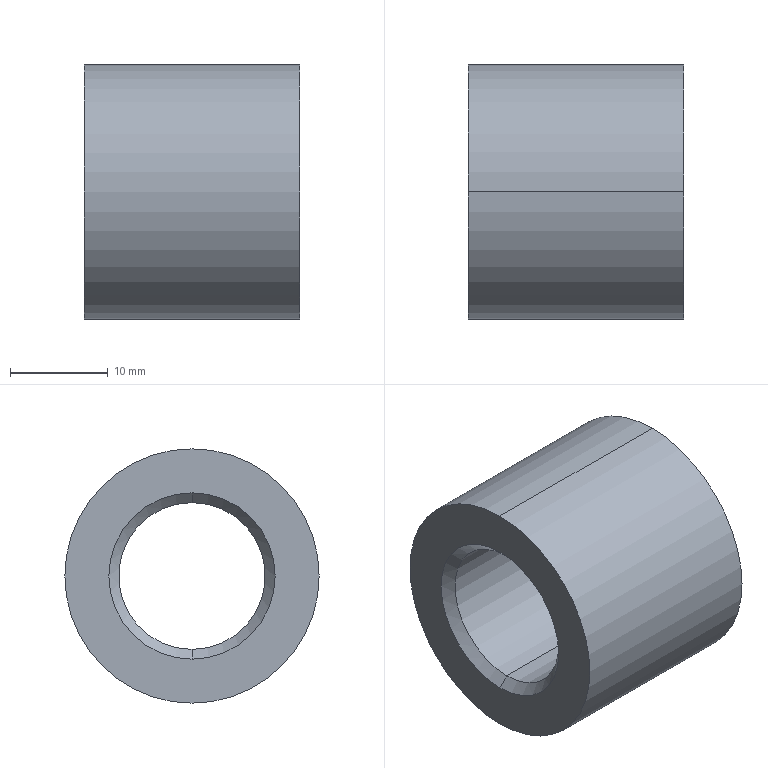Part | SolidWorks | features BaseBody 1 | 1 solid | 10 faces | box 22 x 26 x 26 mm | volume 7744 mm3 | cylinder 4 | cone 4 | plane 2 | commonest cylinder face diameters 15 x2 26 x2
STEP:
#1=CARTESIAN_POINT('',(22.,0.,-13.));
#2=VERTEX_POINT('',#1);
#3=CARTESIAN_POINT('',(22.,0.,13.));
#4=VERTEX_POINT('',#3);
#5=CARTESIAN_POINT('',(22.,0.,0.));
#6=DIRECTION('',(-1.,0.,0.));
#7=DIRECTION('',(0.,1.,0.));
#8=AXIS2_PLACEMENT_3D('',#5,#6,#7);
#9=CIRCLE('',#8,13.);
#10=EDGE_CURVE('',#2,#4,#9,.T.);
#11=ORIENTED_EDGE('',*,*,#10,.T.);
#12=CARTESIAN_POINT('',(0.,0.,13.));
#13=VERTEX_POINT('',#12);
#14=CARTESIAN_POINT('',(22.,0.,13.));
#15=DIRECTION('',(-1.,0.,0.));
#16=VECTOR('',#15,1000.);
#17=LINE('',#14,#16);
#18=EDGE_CURVE('',#4,#13,#17,.T.);
#19=ORIENTED_EDGE('',*,*,#18,.T.);
#20=CARTESIAN_POINT('',(0.,0.,-13.));
#21=VERTEX_POINT('',#20);
#22=CARTESIAN_POINT('',(0.,0.,0.));
#23=DIRECTION('',(-1.,0.,0.));
#24=DIRECTION('',(0.,1.,0.));
#25=AXIS2_PLACEMENT_3D('',#22,#23,#24);
#26=CIRCLE('',#25,13.);
#27=EDGE_CURVE('',#21,#13,#26,.T.);
#28=ORIENTED_EDGE('',*,*,#27,.F.);
#29=CARTESIAN_POINT('',(22.,0.,-13.));
#30=DIRECTION('',(-1.,0.,0.));
#31=VECTOR('',#30,1000.);
#32=LINE('',#29,#31);
#33=EDGE_CURVE('',#2,#21,#32,.T.);
#34=ORIENTED_EDGE('',*,*,#33,.F.);
#35=EDGE_LOOP('',(#11,#19,#28,#34));
#36=FACE_OUTER_BOUND('',#35,.T.);
#37=CARTESIAN_POINT('',(22.,0.,0.));
#38=DIRECTION('',(-1.,0.,0.));
#39=DIRECTION('',(0.,0.,-1.));
#40=AXIS2_PLACEMENT_3D('',#37,#38,#39);
#41=CYLINDRICAL_SURFACE('',#40,13.);
#42=ADVANCED_FACE('',(#36),#41,.T.);
#43=CARTESIAN_POINT('',(21.,0.,-7.5));
#44=VERTEX_POINT('',#43);
#45=CARTESIAN_POINT('',(21.,0.,7.5));
#46=VERTEX_POINT('',#45);
#47=CARTESIAN_POINT('',(21.,0.,0.));
#48=DIRECTION('',(1.,0.,0.));
#49=DIRECTION('',(0.,0.,1.));
#50=AXIS2_PLACEMENT_3D('',#47,#48,#49);
#51=CIRCLE('',#50,7.5);
#52=EDGE_CURVE('',#44,#46,#51,.T.);
#53=ORIENTED_EDGE('',*,*,#52,.T.);
#54=CARTESIAN_POINT('',(1.,0.,7.5));
#55=VERTEX_POINT('',#54);
#56=CARTESIAN_POINT('',(22.,0.,7.5));
#57=DIRECTION('',(-1.,0.,0.));
#58=VECTOR('',#57,1000.);
#59=LINE('',#56,#58);
#60=EDGE_CURVE('',#46,#55,#59,.T.);
#61=ORIENTED_EDGE('',*,*,#60,.T.);
#62=CARTESIAN_POINT('',(1.,0.,-7.5));
#63=VERTEX_POINT('',#62);
#64=CARTESIAN_POINT('',(1.,0.,0.));
#65=DIRECTION('',(-1.,0.,0.));
#66=DIRECTION('',(0.,0.,1.));
#67=AXIS2_PLACEMENT_3D('',#64,#65,#66);
#68=CIRCLE('',#67,7.5);
#69=EDGE_CURVE('',#55,#63,#68,.T.);
#70=ORIENTED_EDGE('',*,*,#69,.T.);
#71=CARTESIAN_POINT('',(22.,0.,-7.5));
#72=DIRECTION('',(-1.,0.,0.));
#73=VECTOR('',#72,1000.);
#74=LINE('',#71,#73);
#75=EDGE_CURVE('',#44,#63,#74,.T.);
#76=ORIENTED_EDGE('',*,*,#75,.F.);
#77=EDGE_LOOP('',(#53,#61,#70,#76));
#78=FACE_OUTER_BOUND('',#77,.T.);
#79=CARTESIAN_POINT('',(22.,0.,0.));
#80=DIRECTION('',(-1.,0.,0.));
#81=DIRECTION('',(0.,0.,-1.));
#82=AXIS2_PLACEMENT_3D('',#79,#80,#81);
#83=CYLINDRICAL_SURFACE('',#82,7.5);
#84=ADVANCED_FACE('',(#78),#83,.F.);
#85=ORIENTED_EDGE('',*,*,#69,.F.);
#86=CARTESIAN_POINT('',(0.,0.,8.5));
#87=VERTEX_POINT('',#86);
#88=CARTESIAN_POINT('',(1.,0.,7.5));
#89=DIRECTION('',(-0.7071,0.,0.7071));
#90=VECTOR('',#89,1000.);
#91=LINE('',#88,#90);
#92=EDGE_CURVE('',#55,#87,#91,.T.);
#93=ORIENTED_EDGE('',*,*,#92,.T.);
#94=CARTESIAN_POINT('',(0.,0.,-8.5));
#95=VERTEX_POINT('',#94);
#96=CARTESIAN_POINT('',(0.,0.,0.));
#97=DIRECTION('',(1.,0.,0.));
#98=DIRECTION('',(0.,0.,1.));
#99=AXIS2_PLACEMENT_3D('',#96,#97,#98);
#100=CIRCLE('',#99,8.5);
#101=EDGE_CURVE('',#95,#87,#100,.T.);
#102=ORIENTED_EDGE('',*,*,#101,.F.);
#103=CARTESIAN_POINT('',(1.,0.,-7.5));
#104=DIRECTION('',(-0.7071,0.,-0.7071));
#105=VECTOR('',#104,1000.);
#106=LINE('',#103,#105);
#107=EDGE_CURVE('',#63,#95,#106,.T.);
#108=ORIENTED_EDGE('',*,*,#107,.F.);
#109=EDGE_LOOP('',(#85,#93,#102,#108));
#110=FACE_OUTER_BOUND('',#109,.T.);
#111=CARTESIAN_POINT('',(1.,0.,0.));
#112=DIRECTION('',(-1.,0.,0.));
#113=DIRECTION('',(0.,0.,-1.));
#114=AXIS2_PLACEMENT_3D('',#111,#112,#113);
#115=CONICAL_SURFACE('',#114,7.5,0.7854);
#116=ADVANCED_FACE('',(#110),#115,.F.);
#117=ORIENTED_EDGE('',*,*,#52,.F.);
#118=CARTESIAN_POINT('',(22.,0.,-8.5));
#119=VERTEX_POINT('',#118);
#120=CARTESIAN_POINT('',(22.,0.,-8.5));
#121=DIRECTION('',(0.7071,0.,-0.7071));
#122=VECTOR('',#121,1000.);
#123=LINE('',#120,#122);
#124=EDGE_CURVE('',#44,#119,#123,.T.);
#125=ORIENTED_EDGE('',*,*,#124,.T.);
#126=CARTESIAN_POINT('',(22.,0.,8.5));
#127=VERTEX_POINT('',#126);
#128=CARTESIAN_POINT('',(22.,0.,0.));
#129=DIRECTION('',(-1.,0.,0.));
#130=DIRECTION('',(0.,0.,1.));
#131=AXIS2_PLACEMENT_3D('',#128,#129,#130);
#132=CIRCLE('',#131,8.5);
#133=EDGE_CURVE('',#127,#119,#132,.T.);
#134=ORIENTED_EDGE('',*,*,#133,.F.);
#135=CARTESIAN_POINT('',(22.,0.,8.5));
#136=DIRECTION('',(0.7071,0.,0.7071));
#137=VECTOR('',#136,1000.);
#138=LINE('',#135,#137);
#139=EDGE_CURVE('',#46,#127,#138,.T.);
#140=ORIENTED_EDGE('',*,*,#139,.F.);
#141=EDGE_LOOP('',(#117,#125,#134,#140));
#142=FACE_OUTER_BOUND('',#141,.T.);
#143=CARTESIAN_POINT('',(22.,0.,0.));
#144=DIRECTION('',(1.,0.,0.));
#145=DIRECTION('',(0.,0.,1.));
#146=AXIS2_PLACEMENT_3D('',#143,#144,#145);
#147=CONICAL_SURFACE('',#146,8.5,0.7854);
#148=ADVANCED_FACE('',(#142),#147,.F.);
#149=ORIENTED_EDGE('',*,*,#124,.F.);
#150=CARTESIAN_POINT('',(21.,0.,0.));
#151=DIRECTION('',(1.,0.,0.));
#152=DIRECTION('',(0.,0.,1.));
#153=AXIS2_PLACEMENT_3D('',#150,#151,#152);
#154=CIRCLE('',#153,7.5);
#155=EDGE_CURVE('',#46,#44,#154,.T.);
#156=ORIENTED_EDGE('',*,*,#155,.F.);
#157=ORIENTED_EDGE('',*,*,#139,.T.);
#158=CARTESIAN_POINT('',(22.,0.,0.));
#159=DIRECTION('',(-1.,0.,0.));
#160=DIRECTION('',(0.,0.,1.));
#161=AXIS2_PLACEMENT_3D('',#158,#159,#160);
#162=CIRCLE('',#161,8.5);
#163=EDGE_CURVE('',#119,#127,#162,.T.);
#164=ORIENTED_EDGE('',*,*,#163,.F.);
#165=EDGE_LOOP('',(#149,#156,#157,#164));
#166=FACE_OUTER_BOUND('',#165,.T.);
#167=CARTESIAN_POINT('',(22.,0.,0.));
#168=DIRECTION('',(1.,0.,0.));
#169=DIRECTION('',(0.,0.,1.));
#170=AXIS2_PLACEMENT_3D('',#167,#168,#169);
#171=CONICAL_SURFACE('',#170,8.5,0.7854);
#172=ADVANCED_FACE('',(#166),#171,.F.);
#173=ORIENTED_EDGE('',*,*,#92,.F.);
#174=CARTESIAN_POINT('',(1.,0.,0.));
#175=DIRECTION('',(-1.,0.,0.));
#176=DIRECTION('',(0.,0.,1.));
#177=AXIS2_PLACEMENT_3D('',#174,#175,#176);
#178=CIRCLE('',#177,7.5);
#179=EDGE_CURVE('',#63,#55,#178,.T.);
#180=ORIENTED_EDGE('',*,*,#179,.F.);
#181=ORIENTED_EDGE('',*,*,#107,.T.);
#182=CARTESIAN_POINT('',(0.,0.,0.));
#183=DIRECTION('',(1.,0.,0.));
#184=DIRECTION('',(0.,0.,1.));
#185=AXIS2_PLACEMENT_3D('',#182,#183,#184);
#186=CIRCLE('',#185,8.5);
#187=EDGE_CURVE('',#87,#95,#186,.T.);
#188=ORIENTED_EDGE('',*,*,#187,.F.);
#189=EDGE_LOOP('',(#173,#180,#181,#188));
#190=FACE_OUTER_BOUND('',#189,.T.);
#191=CARTESIAN_POINT('',(1.,0.,0.));
#192=DIRECTION('',(-1.,0.,0.));
#193=DIRECTION('',(0.,0.,-1.));
#194=AXIS2_PLACEMENT_3D('',#191,#192,#193);
#195=CONICAL_SURFACE('',#194,7.5,0.7854);
#196=ADVANCED_FACE('',(#190),#195,.F.);
#197=ORIENTED_EDGE('',*,*,#27,.T.);
#198=CARTESIAN_POINT('',(0.,0.,0.));
#199=DIRECTION('',(-1.,0.,0.));
#200=DIRECTION('',(0.,1.,0.));
#201=AXIS2_PLACEMENT_3D('',#198,#199,#200);
#202=CIRCLE('',#201,13.);
#203=EDGE_CURVE('',#13,#21,#202,.T.);
#204=ORIENTED_EDGE('',*,*,#203,.T.);
#205=EDGE_LOOP('',(#197,#204));
#206=FACE_OUTER_BOUND('',#205,.T.);
#207=ORIENTED_EDGE('',*,*,#101,.T.);
#208=ORIENTED_EDGE('',*,*,#187,.T.);
#209=EDGE_LOOP('',(#207,#208));
#210=FACE_BOUND('',#209,.T.);
#211=CARTESIAN_POINT('',(0.,0.,0.));
#212=DIRECTION('',(-1.,0.,0.));
#213=DIRECTION('',(0.,0.,1.));
#214=AXIS2_PLACEMENT_3D('',#211,#212,#213);
#215=PLANE('',#214);
#216=ADVANCED_FACE('',(#206,#210),#215,.T.);
#217=ORIENTED_EDGE('',*,*,#10,.F.);
#218=CARTESIAN_POINT('',(22.,0.,0.));
#219=DIRECTION('',(-1.,0.,0.));
#220=DIRECTION('',(0.,1.,0.));
#221=AXIS2_PLACEMENT_3D('',#218,#219,#220);
#222=CIRCLE('',#221,13.);
#223=EDGE_CURVE('',#4,#2,#222,.T.);
#224=ORIENTED_EDGE('',*,*,#223,.F.);
#225=EDGE_LOOP('',(#217,#224));
#226=FACE_OUTER_BOUND('',#225,.T.);
#227=ORIENTED_EDGE('',*,*,#133,.T.);
#228=ORIENTED_EDGE('',*,*,#163,.T.);
#229=EDGE_LOOP('',(#227,#228));
#230=FACE_BOUND('',#229,.T.);
#231=CARTESIAN_POINT('',(22.,0.,0.));
#232=DIRECTION('',(-1.,0.,0.));
#233=DIRECTION('',(0.,0.,1.));
#234=AXIS2_PLACEMENT_3D('',#231,#232,#233);
#235=PLANE('',#234);
#236=ADVANCED_FACE('',(#226,#230),#235,.F.);
#237=ORIENTED_EDGE('',*,*,#60,.F.);
#238=ORIENTED_EDGE('',*,*,#155,.T.);
#239=ORIENTED_EDGE('',*,*,#75,.T.);
#240=ORIENTED_EDGE('',*,*,#179,.T.);
#241=EDGE_LOOP('',(#237,#238,#239,#240));
#242=FACE_OUTER_BOUND('',#241,.T.);
#243=CARTESIAN_POINT('',(22.,0.,0.));
#244=DIRECTION('',(-1.,0.,0.));
#245=DIRECTION('',(0.,0.,-1.));
#246=AXIS2_PLACEMENT_3D('',#243,#244,#245);
#247=CYLINDRICAL_SURFACE('',#246,7.5);
#248=ADVANCED_FACE('',(#242),#247,.F.);
#249=ORIENTED_EDGE('',*,*,#18,.F.);
#250=ORIENTED_EDGE('',*,*,#223,.T.);
#251=ORIENTED_EDGE('',*,*,#33,.T.);
#252=ORIENTED_EDGE('',*,*,#203,.F.);
#253=EDGE_LOOP('',(#249,#250,#251,#252));
#254=FACE_OUTER_BOUND('',#253,.T.);
#255=CARTESIAN_POINT('',(22.,0.,0.));
#256=DIRECTION('',(-1.,0.,0.));
#257=DIRECTION('',(0.,0.,-1.));
#258=AXIS2_PLACEMENT_3D('',#255,#256,#257);
#259=CYLINDRICAL_SURFACE('',#258,13.);
#260=ADVANCED_FACE('',(#254),#259,.T.);
#261=CLOSED_SHELL('',(#42,#84,#116,#148,#172,#196,#216,#236,#248,#260));
#262=MANIFOLD_SOLID_BREP('',#261);
#263=CARTESIAN_POINT('',(0.,0.,0.));
#264=DIRECTION('',(0.,0.,1.));
#265=DIRECTION('',(1.,0.,0.));
#266=AXIS2_PLACEMENT_3D('',#263,#264,#265);
#267=(LENGTH_UNIT()NAMED_UNIT(*)SI_UNIT(.MILLI.,.METRE.));
#268=UNCERTAINTY_MEASURE_WITH_UNIT(LENGTH_MEASURE(0.00001),#267,'','');
#269=(NAMED_UNIT(*)PLANE_ANGLE_UNIT()SI_UNIT($,.RADIAN.));
#270=(NAMED_UNIT(*)SI_UNIT($,.STERADIAN.)SOLID_ANGLE_UNIT());
#271=(GEOMETRIC_REPRESENTATION_CONTEXT(3)GLOBAL_UNCERTAINTY_ASSIGNED_CONTEXT((#268))GLOBAL_UNIT_ASSIGNED_CONTEXT((#267,#269,#270))REPRESENTATION_CONTEXT('',''));
#272=ADVANCED_BREP_SHAPE_REPRESENTATION('',(#262,#266),#271);